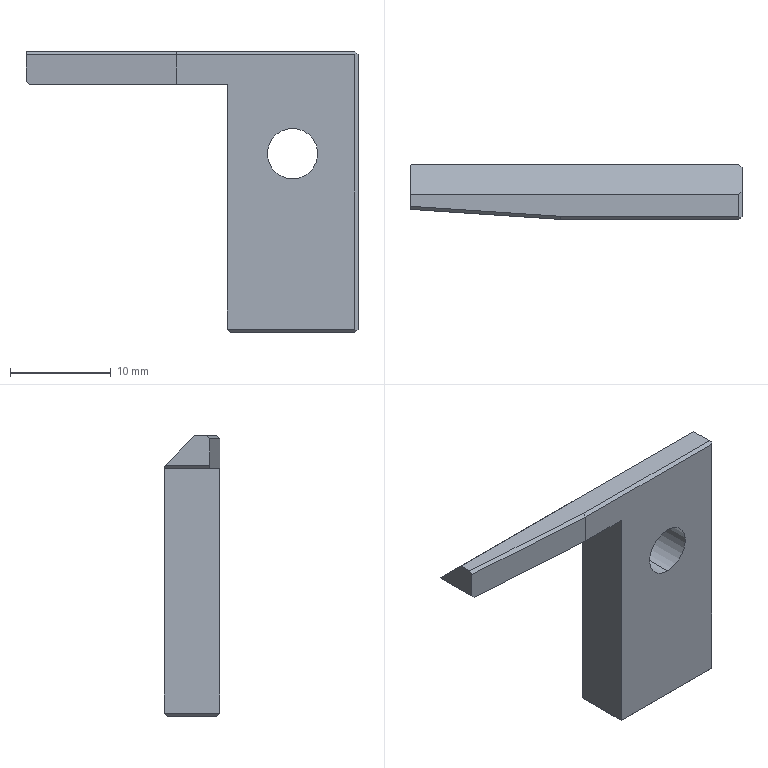Part | NX | 1 solid | 24 faces | box 33 x 5.5 x 27.85 mm | volume 2057 mm3 | plane 20 | cylinder 2 | cone 2 | commonest cylinder face diameters 5 x2
STEP:
#1=CARTESIAN_POINT('',(-176.3,222.248,-74.));
#2=VERTEX_POINT('',#1);
#3=CARTESIAN_POINT('',(-188.7,222.248,-74.));
#4=VERTEX_POINT('',#3);
#5=CARTESIAN_POINT('',(-182.5,222.248,-74.));
#6=DIRECTION('',(-1.,0.,0.));
#7=VECTOR('',#6,1000.);
#8=LINE('',#5,#7);
#9=EDGE_CURVE('',#2,#4,#8,.T.);
#10=ORIENTED_EDGE('',*,*,#9,.T.);
#11=CARTESIAN_POINT('',(-188.7,227.148,-74.));
#12=VERTEX_POINT('',#11);
#13=CARTESIAN_POINT('',(-188.7,224.698,-74.));
#14=DIRECTION('',(0.,-1.,0.));
#15=VECTOR('',#14,1000.);
#16=LINE('',#13,#15);
#17=EDGE_CURVE('',#12,#4,#16,.T.);
#18=ORIENTED_EDGE('',*,*,#17,.F.);
#19=CARTESIAN_POINT('',(-176.3,227.148,-74.));
#20=VERTEX_POINT('',#19);
#21=CARTESIAN_POINT('',(-182.5,227.148,-74.));
#22=DIRECTION('',(1.,0.,0.));
#23=VECTOR('',#22,1000.);
#24=LINE('',#21,#23);
#25=EDGE_CURVE('',#12,#20,#24,.T.);
#26=ORIENTED_EDGE('',*,*,#25,.T.);
#27=CARTESIAN_POINT('',(-176.3,224.698,-74.));
#28=DIRECTION('',(0.,-1.,0.));
#29=VECTOR('',#28,1000.);
#30=LINE('',#27,#29);
#31=EDGE_CURVE('',#20,#2,#30,.T.);
#32=ORIENTED_EDGE('',*,*,#31,.T.);
#33=EDGE_LOOP('',(#10,#18,#26,#32));
#34=FACE_BOUND('',#33,.T.);
#35=CARTESIAN_POINT('',(-175.,217.7,-74.));
#36=DIRECTION('',(0.,0.,-1.));
#37=DIRECTION('',(-1.,0.,0.));
#38=AXIS2_PLACEMENT_3D('',#35,#36,#37);
#39=PLANE('',#38);
#40=ADVANCED_FACE('',(#34),#39,.T.);
#41=CARTESIAN_POINT('',(-209.,227.348,-49.05));
#42=VERTEX_POINT('',#41);
#43=CARTESIAN_POINT('',(-209.,222.948,-49.05));
#44=VERTEX_POINT('',#43);
#45=CARTESIAN_POINT('',(-209.,225.198,-49.05));
#46=DIRECTION('',(0.,-1.,0.));
#47=VECTOR('',#46,1000.);
#48=LINE('',#45,#47);
#49=EDGE_CURVE('',#42,#44,#48,.T.);
#50=ORIENTED_EDGE('',*,*,#49,.T.);
#51=CARTESIAN_POINT('',(-209.,222.948,-46.45));
#52=VERTEX_POINT('',#51);
#53=CARTESIAN_POINT('',(-209.,222.948,-47.75));
#54=DIRECTION('',(0.,0.,-1.));
#55=VECTOR('',#54,1000.);
#56=LINE('',#53,#55);
#57=EDGE_CURVE('',#52,#44,#56,.T.);
#58=ORIENTED_EDGE('',*,*,#57,.F.);
#59=CARTESIAN_POINT('',(-209.,223.249,-46.15));
#60=VERTEX_POINT('',#59);
#61=CARTESIAN_POINT('',(-209.,213.364,-56.013));
#62=DIRECTION('',(0.,-0.7079,-0.7063));
#63=VECTOR('',#62,1000.);
#64=LINE('',#61,#63);
#65=EDGE_CURVE('',#60,#52,#64,.T.);
#66=ORIENTED_EDGE('',*,*,#65,.F.);
#67=CARTESIAN_POINT('',(-209.,224.448,-46.15));
#68=VERTEX_POINT('',#67);
#69=CARTESIAN_POINT('',(-209.,213.364,-46.15));
#70=DIRECTION('',(0.,1.,0.));
#71=VECTOR('',#70,1000.);
#72=LINE('',#69,#71);
#73=EDGE_CURVE('',#60,#68,#72,.T.);
#74=ORIENTED_EDGE('',*,*,#73,.T.);
#75=CARTESIAN_POINT('',(-209.,232.274,-53.975));
#76=DIRECTION('',(0.,0.7071,-0.7071));
#77=VECTOR('',#76,1000.);
#78=LINE('',#75,#77);
#79=EDGE_CURVE('',#68,#42,#78,.T.);
#80=ORIENTED_EDGE('',*,*,#79,.T.);
#81=EDGE_LOOP('',(#50,#58,#66,#74,#80));
#82=FACE_BOUND('',#81,.T.);
#83=CARTESIAN_POINT('',(-209.,224.834,-50.132));
#84=DIRECTION('',(-1.,0.,0.));
#85=DIRECTION('',(0.,0.,1.));
#86=AXIS2_PLACEMENT_3D('',#83,#84,#85);
#87=PLANE('',#86);
#88=ADVANCED_FACE('',(#82),#87,.T.);
#89=CARTESIAN_POINT('',(-176.3,227.448,-73.7));
#90=VERTEX_POINT('',#89);
#91=CARTESIAN_POINT('',(-176.3,227.448,-49.15));
#92=VERTEX_POINT('',#91);
#93=CARTESIAN_POINT('',(-176.3,227.448,-61.575));
#94=DIRECTION('',(0.,0.,1.));
#95=VECTOR('',#94,1000.);
#96=LINE('',#93,#95);
#97=EDGE_CURVE('',#90,#92,#96,.T.);
#98=ORIENTED_EDGE('',*,*,#97,.F.);
#99=CARTESIAN_POINT('',(-189.,227.448,-73.7));
#100=VERTEX_POINT('',#99);
#101=CARTESIAN_POINT('',(-182.5,227.448,-73.7));
#102=DIRECTION('',(1.,0.,0.));
#103=VECTOR('',#102,1000.);
#104=LINE('',#101,#103);
#105=EDGE_CURVE('',#100,#90,#104,.T.);
#106=ORIENTED_EDGE('',*,*,#105,.F.);
#107=CARTESIAN_POINT('',(-189.,227.448,-49.35));
#108=VERTEX_POINT('',#107);
#109=CARTESIAN_POINT('',(-189.,227.448,-53.975));
#110=DIRECTION('',(0.,0.,1.));
#111=VECTOR('',#110,1000.);
#112=LINE('',#109,#111);
#113=EDGE_CURVE('',#100,#108,#112,.T.);
#114=ORIENTED_EDGE('',*,*,#113,.T.);
#115=CARTESIAN_POINT('',(-208.7,227.448,-49.35));
#116=VERTEX_POINT('',#115);
#117=CARTESIAN_POINT('',(-175.,227.448,-49.35));
#118=DIRECTION('',(1.,0.,0.));
#119=VECTOR('',#118,1000.);
#120=LINE('',#117,#119);
#121=EDGE_CURVE('',#116,#108,#120,.T.);
#122=ORIENTED_EDGE('',*,*,#121,.F.);
#123=CARTESIAN_POINT('',(-208.9,227.448,-49.15));
#124=VERTEX_POINT('',#123);
#125=CARTESIAN_POINT('',(-204.075,227.448,-53.975));
#126=DIRECTION('',(0.7071,0.,-0.7071));
#127=VECTOR('',#126,1000.);
#128=LINE('',#125,#127);
#129=EDGE_CURVE('',#124,#116,#128,.T.);
#130=ORIENTED_EDGE('',*,*,#129,.F.);
#131=CARTESIAN_POINT('',(-192.5,227.448,-49.15));
#132=DIRECTION('',(1.,0.,0.));
#133=VECTOR('',#132,1000.);
#134=LINE('',#131,#133);
#135=EDGE_CURVE('',#124,#92,#134,.T.);
#136=ORIENTED_EDGE('',*,*,#135,.T.);
#137=EDGE_LOOP('',(#98,#106,#114,#122,#130,#136));
#138=FACE_BOUND('',#137,.T.);
#139=CARTESIAN_POINT('',(-182.5,227.448,-53.563));
#140=VERTEX_POINT('',#139);
#141=CARTESIAN_POINT('',(-182.5,227.448,-58.963));
#142=VERTEX_POINT('',#141);
#143=CARTESIAN_POINT('',(-182.5,227.448,-56.263));
#144=DIRECTION('',(0.,1.,0.));
#145=DIRECTION('',(0.,0.,-1.));
#146=AXIS2_PLACEMENT_3D('',#143,#144,#145);
#147=CIRCLE('',#146,2.7);
#148=EDGE_CURVE('',#140,#142,#147,.T.);
#149=ORIENTED_EDGE('',*,*,#148,.F.);
#150=CARTESIAN_POINT('',(-182.5,227.448,-56.263));
#151=DIRECTION('',(0.,1.,0.));
#152=DIRECTION('',(0.,0.,-1.));
#153=AXIS2_PLACEMENT_3D('',#150,#151,#152);
#154=CIRCLE('',#153,2.7);
#155=EDGE_CURVE('',#142,#140,#154,.T.);
#156=ORIENTED_EDGE('',*,*,#155,.F.);
#157=EDGE_LOOP('',(#149,#156));
#158=FACE_BOUND('',#157,.T.);
#159=CARTESIAN_POINT('',(-175.,227.448,-64.15));
#160=DIRECTION('',(0.,1.,0.));
#161=DIRECTION('',(0.,0.,-1.));
#162=AXIS2_PLACEMENT_3D('',#159,#160,#161);
#163=PLANE('',#162);
#164=ADVANCED_FACE('',(#138,#158),#163,.T.);
#165=CARTESIAN_POINT('',(-176.3,222.248,-46.15));
#166=VERTEX_POINT('',#165);
#167=CARTESIAN_POINT('',(-193.99,222.248,-46.15));
#168=VERTEX_POINT('',#167);
#169=CARTESIAN_POINT('',(-185.,222.248,-46.15));
#170=DIRECTION('',(-1.,0.,0.));
#171=VECTOR('',#170,1000.);
#172=LINE('',#169,#171);
#173=EDGE_CURVE('',#166,#168,#172,.T.);
#174=ORIENTED_EDGE('',*,*,#173,.F.);
#175=CARTESIAN_POINT('',(-176.3,224.448,-46.15));
#176=VERTEX_POINT('',#175);
#177=CARTESIAN_POINT('',(-176.3,223.198,-46.15));
#178=DIRECTION('',(0.,-1.,0.));
#179=VECTOR('',#178,1000.);
#180=LINE('',#177,#179);
#181=EDGE_CURVE('',#176,#166,#180,.T.);
#182=ORIENTED_EDGE('',*,*,#181,.F.);
#183=CARTESIAN_POINT('',(-192.5,224.448,-46.15));
#184=DIRECTION('',(1.,0.,0.));
#185=VECTOR('',#184,1000.);
#186=LINE('',#183,#185);
#187=EDGE_CURVE('',#68,#176,#186,.T.);
#188=ORIENTED_EDGE('',*,*,#187,.F.);
#189=ORIENTED_EDGE('',*,*,#73,.F.);
#190=CARTESIAN_POINT('',(-201.48,222.747,-46.15));
#191=DIRECTION('',(-0.9978,0.06652,0.));
#192=VECTOR('',#191,1000.);
#193=LINE('',#190,#192);
#194=EDGE_CURVE('',#168,#60,#193,.T.);
#195=ORIENTED_EDGE('',*,*,#194,.F.);
#196=EDGE_LOOP('',(#174,#182,#188,#189,#195));
#197=FACE_BOUND('',#196,.T.);
#198=CARTESIAN_POINT('',(-175.,222.398,-46.15));
#199=DIRECTION('',(0.,0.,1.));
#200=DIRECTION('',(1.,0.,0.));
#201=AXIS2_PLACEMENT_3D('',#198,#199,#200);
#202=PLANE('',#201);
#203=ADVANCED_FACE('',(#197),#202,.T.);
#204=CARTESIAN_POINT('',(-194.,221.948,-49.35));
#205=VERTEX_POINT('',#204);
#206=CARTESIAN_POINT('',(-189.,221.948,-49.35));
#207=VERTEX_POINT('',#206);
#208=CARTESIAN_POINT('',(-175.,221.948,-49.35));
#209=DIRECTION('',(1.,0.,0.));
#210=VECTOR('',#209,1000.);
#211=LINE('',#208,#210);
#212=EDGE_CURVE('',#205,#207,#211,.T.);
#213=ORIENTED_EDGE('',*,*,#212,.F.);
#214=CARTESIAN_POINT('',(-208.7,222.928,-49.35));
#215=VERTEX_POINT('',#214);
#216=CARTESIAN_POINT('',(-175.,220.681,-49.35));
#217=DIRECTION('',(0.9978,-0.06652,0.));
#218=VECTOR('',#217,1000.);
#219=LINE('',#216,#218);
#220=EDGE_CURVE('',#215,#205,#219,.T.);
#221=ORIENTED_EDGE('',*,*,#220,.F.);
#222=CARTESIAN_POINT('',(-208.7,225.198,-49.35));
#223=DIRECTION('',(0.,-1.,0.));
#224=VECTOR('',#223,1000.);
#225=LINE('',#222,#224);
#226=EDGE_CURVE('',#116,#215,#225,.T.);
#227=ORIENTED_EDGE('',*,*,#226,.F.);
#228=ORIENTED_EDGE('',*,*,#121,.T.);
#229=CARTESIAN_POINT('',(-189.,213.364,-49.35));
#230=DIRECTION('',(0.,1.,0.));
#231=VECTOR('',#230,1000.);
#232=LINE('',#229,#231);
#233=EDGE_CURVE('',#207,#108,#232,.T.);
#234=ORIENTED_EDGE('',*,*,#233,.F.);
#235=EDGE_LOOP('',(#213,#221,#227,#228,#234));
#236=FACE_BOUND('',#235,.T.);
#237=CARTESIAN_POINT('',(-189.,221.948,-49.35));
#238=DIRECTION('',(0.,0.,-1.));
#239=DIRECTION('',(-1.,0.,0.));
#240=AXIS2_PLACEMENT_3D('',#237,#238,#239);
#241=PLANE('',#240);
#242=ADVANCED_FACE('',(#236),#241,.T.);
#243=CARTESIAN_POINT('',(-176.3,221.948,-46.45));
#244=VERTEX_POINT('',#243);
#245=CARTESIAN_POINT('',(-194.,221.948,-46.45));
#246=VERTEX_POINT('',#245);
#247=CARTESIAN_POINT('',(-185.,221.948,-46.45));
#248=DIRECTION('',(-1.,0.,0.));
#249=VECTOR('',#248,1000.);
#250=LINE('',#247,#249);
#251=EDGE_CURVE('',#244,#246,#250,.T.);
#252=ORIENTED_EDGE('',*,*,#251,.T.);
#253=CARTESIAN_POINT('',(-194.,221.948,-47.75));
#254=DIRECTION('',(0.,0.,-1.));
#255=VECTOR('',#254,1000.);
#256=LINE('',#253,#255);
#257=EDGE_CURVE('',#246,#205,#256,.T.);
#258=ORIENTED_EDGE('',*,*,#257,.T.);
#259=ORIENTED_EDGE('',*,*,#212,.T.);
#260=CARTESIAN_POINT('',(-189.,221.948,-73.7));
#261=VERTEX_POINT('',#260);
#262=CARTESIAN_POINT('',(-189.,221.948,-53.975));
#263=DIRECTION('',(0.,0.,-1.));
#264=VECTOR('',#263,1000.);
#265=LINE('',#262,#264);
#266=EDGE_CURVE('',#207,#261,#265,.T.);
#267=ORIENTED_EDGE('',*,*,#266,.T.);
#268=CARTESIAN_POINT('',(-176.3,221.948,-73.7));
#269=VERTEX_POINT('',#268);
#270=CARTESIAN_POINT('',(-182.5,221.948,-73.7));
#271=DIRECTION('',(-1.,0.,0.));
#272=VECTOR('',#271,1000.);
#273=LINE('',#270,#272);
#274=EDGE_CURVE('',#269,#261,#273,.T.);
#275=ORIENTED_EDGE('',*,*,#274,.F.);
#276=CARTESIAN_POINT('',(-176.3,221.948,-60.075));
#277=DIRECTION('',(0.,0.,1.));
#278=VECTOR('',#277,1000.);
#279=LINE('',#276,#278);
#280=EDGE_CURVE('',#269,#244,#279,.T.);
#281=ORIENTED_EDGE('',*,*,#280,.T.);
#282=EDGE_LOOP('',(#252,#258,#259,#267,#275,#281));
#283=FACE_BOUND('',#282,.T.);
#284=CARTESIAN_POINT('',(-182.5,221.948,-53.763));
#285=VERTEX_POINT('',#284);
#286=CARTESIAN_POINT('',(-182.5,221.948,-58.763));
#287=VERTEX_POINT('',#286);
#288=CARTESIAN_POINT('',(-182.5,221.948,-56.263));
#289=DIRECTION('',(0.,1.,0.));
#290=DIRECTION('',(0.,0.,-1.));
#291=AXIS2_PLACEMENT_3D('',#288,#289,#290);
#292=CIRCLE('',#291,2.5);
#293=EDGE_CURVE('',#285,#287,#292,.T.);
#294=ORIENTED_EDGE('',*,*,#293,.T.);
#295=CARTESIAN_POINT('',(-182.5,221.948,-56.263));
#296=DIRECTION('',(0.,1.,0.));
#297=DIRECTION('',(0.,0.,-1.));
#298=AXIS2_PLACEMENT_3D('',#295,#296,#297);
#299=CIRCLE('',#298,2.5);
#300=EDGE_CURVE('',#287,#285,#299,.T.);
#301=ORIENTED_EDGE('',*,*,#300,.T.);
#302=EDGE_LOOP('',(#294,#301));
#303=FACE_BOUND('',#302,.T.);
#304=CARTESIAN_POINT('',(-189.,221.948,-45.15));
#305=DIRECTION('',(0.,-1.,0.));
#306=DIRECTION('',(-1.,0.,0.));
#307=AXIS2_PLACEMENT_3D('',#304,#305,#306);
#308=PLANE('',#307);
#309=ADVANCED_FACE('',(#283,#303),#308,.T.);
#310=CARTESIAN_POINT('',(-182.5,227.248,-53.763));
#311=VERTEX_POINT('',#310);
#312=CARTESIAN_POINT('',(-182.5,227.248,-58.763));
#313=VERTEX_POINT('',#312);
#314=CARTESIAN_POINT('',(-182.5,227.248,-56.263));
#315=DIRECTION('',(0.,1.,0.));
#316=DIRECTION('',(0.,0.,-1.));
#317=AXIS2_PLACEMENT_3D('',#314,#315,#316);
#318=CIRCLE('',#317,2.5);
#319=EDGE_CURVE('',#311,#313,#318,.T.);
#320=ORIENTED_EDGE('',*,*,#319,.T.);
#321=CARTESIAN_POINT('',(-182.5,227.948,-58.763));
#322=DIRECTION('',(0.,1.,0.));
#323=VECTOR('',#322,1000.);
#324=LINE('',#321,#323);
#325=EDGE_CURVE('',#313,#287,#324,.F.);
#326=ORIENTED_EDGE('',*,*,#325,.T.);
#327=ORIENTED_EDGE('',*,*,#293,.F.);
#328=CARTESIAN_POINT('',(-182.5,227.948,-53.763));
#329=DIRECTION('',(0.,1.,0.));
#330=VECTOR('',#329,1000.);
#331=LINE('',#328,#330);
#332=EDGE_CURVE('',#311,#285,#331,.F.);
#333=ORIENTED_EDGE('',*,*,#332,.F.);
#334=EDGE_LOOP('',(#320,#326,#327,#333));
#335=FACE_BOUND('',#334,.T.);
#336=CARTESIAN_POINT('',(-182.5,227.948,-56.263));
#337=DIRECTION('',(0.,1.,0.));
#338=DIRECTION('',(0.,0.,-1.));
#339=AXIS2_PLACEMENT_3D('',#336,#337,#338);
#340=CYLINDRICAL_SURFACE('',#339,2.5);
#341=ADVANCED_FACE('',(#335),#340,.F.);
#342=ORIENTED_EDGE('',*,*,#187,.T.);
#343=CARTESIAN_POINT('',(-176.,224.748,-46.45));
#344=VERTEX_POINT('',#343);
#345=CARTESIAN_POINT('',(-175.,225.748,-47.45));
#346=DIRECTION('',(0.5774,0.5774,-0.5774));
#347=VECTOR('',#346,1000.);
#348=LINE('',#345,#347);
#349=EDGE_CURVE('',#176,#344,#348,.T.);
#350=ORIENTED_EDGE('',*,*,#349,.T.);
#351=CARTESIAN_POINT('',(-176.,227.148,-48.85));
#352=VERTEX_POINT('',#351);
#353=CARTESIAN_POINT('',(-176.,232.274,-53.975));
#354=DIRECTION('',(0.,-0.7071,0.7071));
#355=VECTOR('',#354,1000.);
#356=LINE('',#353,#355);
#357=EDGE_CURVE('',#352,#344,#356,.T.);
#358=ORIENTED_EDGE('',*,*,#357,.F.);
#359=CARTESIAN_POINT('',(-181.125,232.274,-53.975));
#360=DIRECTION('',(-0.5774,0.5774,-0.5774));
#361=VECTOR('',#360,1000.);
#362=LINE('',#359,#361);
#363=EDGE_CURVE('',#352,#92,#362,.T.);
#364=ORIENTED_EDGE('',*,*,#363,.T.);
#365=ORIENTED_EDGE('',*,*,#135,.F.);
#366=CARTESIAN_POINT('',(-204.075,232.274,-53.975));
#367=DIRECTION('',(-0.5774,-0.5774,0.5774));
#368=VECTOR('',#367,1000.);
#369=LINE('',#366,#368);
#370=EDGE_CURVE('',#124,#42,#369,.T.);
#371=ORIENTED_EDGE('',*,*,#370,.T.);
#372=ORIENTED_EDGE('',*,*,#79,.F.);
#373=EDGE_LOOP('',(#342,#350,#358,#364,#365,#371,#372));
#374=FACE_BOUND('',#373,.T.);
#375=CARTESIAN_POINT('',(-192.5,225.948,-47.65));
#376=DIRECTION('',(0.,-0.7071,-0.7071));
#377=DIRECTION('',(0.,0.7071,-0.7071));
#378=AXIS2_PLACEMENT_3D('',#375,#376,#377);
#379=PLANE('',#378);
#380=ADVANCED_FACE('',(#374),#379,.F.);
#381=ORIENTED_EDGE('',*,*,#319,.F.);
#382=CARTESIAN_POINT('',(-182.5,227.248,-53.763));
#383=DIRECTION('',(0.,0.7071,0.7071));
#384=VECTOR('',#383,1000.);
#385=LINE('',#382,#384);
#386=EDGE_CURVE('',#140,#311,#385,.F.);
#387=ORIENTED_EDGE('',*,*,#386,.F.);
#388=ORIENTED_EDGE('',*,*,#148,.T.);
#389=CARTESIAN_POINT('',(-182.5,227.248,-58.763));
#390=DIRECTION('',(0.,0.7071,-0.7071));
#391=VECTOR('',#390,1000.);
#392=LINE('',#389,#391);
#393=EDGE_CURVE('',#142,#313,#392,.F.);
#394=ORIENTED_EDGE('',*,*,#393,.T.);
#395=EDGE_LOOP('',(#381,#387,#388,#394));
#396=FACE_BOUND('',#395,.T.);
#397=CARTESIAN_POINT('',(-182.5,227.248,-56.263));
#398=DIRECTION('',(0.,1.,0.));
#399=DIRECTION('',(0.,0.,-1.));
#400=AXIS2_PLACEMENT_3D('',#397,#398,#399);
#401=CONICAL_SURFACE('',#400,2.5,0.7854);
#402=ADVANCED_FACE('',(#396),#401,.F.);
#403=CARTESIAN_POINT('',(-201.5,222.448,-46.45));
#404=DIRECTION('',(-0.9978,0.06652,0.));
#405=VECTOR('',#404,1000.);
#406=LINE('',#403,#405);
#407=EDGE_CURVE('',#246,#52,#406,.T.);
#408=ORIENTED_EDGE('',*,*,#407,.T.);
#409=ORIENTED_EDGE('',*,*,#57,.T.);
#410=CARTESIAN_POINT('',(-204.075,222.62,-53.975));
#411=DIRECTION('',(-0.7063,0.04709,0.7063));
#412=VECTOR('',#411,1000.);
#413=LINE('',#410,#412);
#414=EDGE_CURVE('',#215,#44,#413,.T.);
#415=ORIENTED_EDGE('',*,*,#414,.F.);
#416=ORIENTED_EDGE('',*,*,#220,.T.);
#417=ORIENTED_EDGE('',*,*,#257,.F.);
#418=EDGE_LOOP('',(#408,#409,#415,#416,#417));
#419=FACE_BOUND('',#418,.T.);
#420=CARTESIAN_POINT('',(-201.5,222.448,-47.75));
#421=DIRECTION('',(-0.06652,-0.9978,0.));
#422=DIRECTION('',(-0.9978,0.06652,0.));
#423=AXIS2_PLACEMENT_3D('',#420,#421,#422);
#424=PLANE('',#423);
#425=ADVANCED_FACE('',(#419),#424,.T.);
#426=ORIENTED_EDGE('',*,*,#25,.F.);
#427=CARTESIAN_POINT('',(-174.916,213.364,-87.784));
#428=DIRECTION('',(-0.5774,0.5774,0.5774));
#429=VECTOR('',#428,1000.);
#430=LINE('',#427,#429);
#431=EDGE_CURVE('',#12,#100,#430,.T.);
#432=ORIENTED_EDGE('',*,*,#431,.T.);
#433=ORIENTED_EDGE('',*,*,#105,.T.);
#434=CARTESIAN_POINT('',(-176.15,227.298,-73.85));
#435=VERTEX_POINT('',#434);
#436=CARTESIAN_POINT('',(-162.216,213.364,-87.784));
#437=DIRECTION('',(-0.5774,0.5774,0.5774));
#438=VECTOR('',#437,1000.);
#439=LINE('',#436,#438);
#440=EDGE_CURVE('',#435,#90,#439,.T.);
#441=ORIENTED_EDGE('',*,*,#440,.F.);
#442=CARTESIAN_POINT('',(-190.084,213.364,-87.784));
#443=DIRECTION('',(0.5774,0.5774,0.5774));
#444=VECTOR('',#443,1000.);
#445=LINE('',#442,#444);
#446=EDGE_CURVE('',#20,#435,#445,.T.);
#447=ORIENTED_EDGE('',*,*,#446,.F.);
#448=EDGE_LOOP('',(#426,#432,#433,#441,#447));
#449=FACE_BOUND('',#448,.T.);
#450=CARTESIAN_POINT('',(-182.5,227.298,-73.85));
#451=DIRECTION('',(0.,0.7071,-0.7071));
#452=DIRECTION('',(-1.,0.,0.));
#453=AXIS2_PLACEMENT_3D('',#450,#451,#452);
#454=PLANE('',#453);
#455=ADVANCED_FACE('',(#449),#454,.T.);
#456=ORIENTED_EDGE('',*,*,#9,.F.);
#457=CARTESIAN_POINT('',(-176.15,222.098,-73.85));
#458=VERTEX_POINT('',#457);
#459=CARTESIAN_POINT('',(-167.416,213.364,-65.116));
#460=DIRECTION('',(0.5774,-0.5774,0.5774));
#461=VECTOR('',#460,1000.);
#462=LINE('',#459,#461);
#463=EDGE_CURVE('',#2,#458,#462,.T.);
#464=ORIENTED_EDGE('',*,*,#463,.T.);
#465=CARTESIAN_POINT('',(-184.884,213.364,-65.116));
#466=DIRECTION('',(0.5774,0.5774,-0.5774));
#467=VECTOR('',#466,1000.);
#468=LINE('',#465,#467);
#469=EDGE_CURVE('',#269,#458,#468,.T.);
#470=ORIENTED_EDGE('',*,*,#469,.F.);
#471=ORIENTED_EDGE('',*,*,#274,.T.);
#472=CARTESIAN_POINT('',(-197.584,213.364,-65.116));
#473=DIRECTION('',(0.5774,0.5774,-0.5774));
#474=VECTOR('',#473,1000.);
#475=LINE('',#472,#474);
#476=EDGE_CURVE('',#261,#4,#475,.T.);
#477=ORIENTED_EDGE('',*,*,#476,.T.);
#478=EDGE_LOOP('',(#456,#464,#470,#471,#477));
#479=FACE_BOUND('',#478,.T.);
#480=CARTESIAN_POINT('',(-182.5,222.098,-73.85));
#481=DIRECTION('',(0.,-0.7071,-0.7071));
#482=DIRECTION('',(0.,-0.7071,0.7071));
#483=AXIS2_PLACEMENT_3D('',#480,#481,#482);
#484=PLANE('',#483);
#485=ADVANCED_FACE('',(#479),#484,.T.);
#486=ORIENTED_EDGE('',*,*,#49,.F.);
#487=ORIENTED_EDGE('',*,*,#370,.F.);
#488=ORIENTED_EDGE('',*,*,#129,.T.);
#489=ORIENTED_EDGE('',*,*,#226,.T.);
#490=ORIENTED_EDGE('',*,*,#414,.T.);
#491=EDGE_LOOP('',(#486,#487,#488,#489,#490));
#492=FACE_BOUND('',#491,.T.);
#493=CARTESIAN_POINT('',(-208.85,225.198,-49.2));
#494=DIRECTION('',(-0.7071,0.,-0.7071));
#495=DIRECTION('',(-0.7071,0.,0.7071));
#496=AXIS2_PLACEMENT_3D('',#493,#494,#495);
#497=PLANE('',#496);
#498=ADVANCED_FACE('',(#492),#497,.T.);
#499=ORIENTED_EDGE('',*,*,#251,.F.);
#500=CARTESIAN_POINT('',(-176.15,222.098,-46.3));
#501=VERTEX_POINT('',#500);
#502=CARTESIAN_POINT('',(-175.,223.248,-45.15));
#503=DIRECTION('',(0.5774,0.5774,0.5774));
#504=VECTOR('',#503,1000.);
#505=LINE('',#502,#504);
#506=EDGE_CURVE('',#244,#501,#505,.T.);
#507=ORIENTED_EDGE('',*,*,#506,.T.);
#508=CARTESIAN_POINT('',(-167.416,213.364,-55.034));
#509=DIRECTION('',(-0.5774,0.5774,0.5774));
#510=VECTOR('',#509,1000.);
#511=LINE('',#508,#510);
#512=EDGE_CURVE('',#501,#166,#511,.T.);
#513=ORIENTED_EDGE('',*,*,#512,.T.);
#514=ORIENTED_EDGE('',*,*,#173,.T.);
#515=CARTESIAN_POINT('',(-194.286,213.364,-55.034));
#516=DIRECTION('',(-0.02354,-0.7069,-0.7069));
#517=VECTOR('',#516,1000.);
#518=LINE('',#515,#517);
#519=EDGE_CURVE('',#168,#246,#518,.T.);
#520=ORIENTED_EDGE('',*,*,#519,.T.);
#521=EDGE_LOOP('',(#499,#507,#513,#514,#520));
#522=FACE_BOUND('',#521,.T.);
#523=CARTESIAN_POINT('',(-185.,222.098,-46.3));
#524=DIRECTION('',(0.,-0.7071,0.7071));
#525=DIRECTION('',(-1.,0.,0.));
#526=AXIS2_PLACEMENT_3D('',#523,#524,#525);
#527=PLANE('',#526);
#528=ADVANCED_FACE('',(#522),#527,.T.);
#529=ORIENTED_EDGE('',*,*,#407,.F.);
#530=ORIENTED_EDGE('',*,*,#519,.F.);
#531=ORIENTED_EDGE('',*,*,#194,.T.);
#532=ORIENTED_EDGE('',*,*,#65,.T.);
#533=EDGE_LOOP('',(#529,#530,#531,#532));
#534=FACE_BOUND('',#533,.T.);
#535=CARTESIAN_POINT('',(-201.49,222.598,-46.3));
#536=DIRECTION('',(-0.04704,-0.7055,0.7071));
#537=DIRECTION('',(-0.9978,0.06652,0.));
#538=AXIS2_PLACEMENT_3D('',#535,#536,#537);
#539=PLANE('',#538);
#540=ADVANCED_FACE('',(#534),#539,.T.);
#541=ORIENTED_EDGE('',*,*,#393,.F.);
#542=ORIENTED_EDGE('',*,*,#155,.T.);
#543=ORIENTED_EDGE('',*,*,#386,.T.);
#544=CARTESIAN_POINT('',(-182.5,227.248,-56.263));
#545=DIRECTION('',(0.,1.,0.));
#546=DIRECTION('',(0.,0.,-1.));
#547=AXIS2_PLACEMENT_3D('',#544,#545,#546);
#548=CIRCLE('',#547,2.5);
#549=EDGE_CURVE('',#313,#311,#548,.T.);
#550=ORIENTED_EDGE('',*,*,#549,.F.);
#551=EDGE_LOOP('',(#541,#542,#543,#550));
#552=FACE_BOUND('',#551,.T.);
#553=CARTESIAN_POINT('',(-182.5,227.248,-56.263));
#554=DIRECTION('',(0.,1.,0.));
#555=DIRECTION('',(0.,0.,-1.));
#556=AXIS2_PLACEMENT_3D('',#553,#554,#555);
#557=CONICAL_SURFACE('',#556,2.5,0.7854);
#558=ADVANCED_FACE('',(#552),#557,.F.);
#559=ORIENTED_EDGE('',*,*,#325,.F.);
#560=ORIENTED_EDGE('',*,*,#549,.T.);
#561=ORIENTED_EDGE('',*,*,#332,.T.);
#562=ORIENTED_EDGE('',*,*,#300,.F.);
#563=EDGE_LOOP('',(#559,#560,#561,#562));
#564=FACE_BOUND('',#563,.T.);
#565=CARTESIAN_POINT('',(-182.5,227.948,-56.263));
#566=DIRECTION('',(0.,1.,0.));
#567=DIRECTION('',(0.,0.,-1.));
#568=AXIS2_PLACEMENT_3D('',#565,#566,#567);
#569=CYLINDRICAL_SURFACE('',#568,2.5);
#570=ADVANCED_FACE('',(#564),#569,.F.);
#571=CARTESIAN_POINT('',(-189.,224.698,-73.7));
#572=DIRECTION('',(0.,-1.,0.));
#573=VECTOR('',#572,1000.);
#574=LINE('',#571,#573);
#575=EDGE_CURVE('',#100,#261,#574,.T.);
#576=ORIENTED_EDGE('',*,*,#575,.T.);
#577=ORIENTED_EDGE('',*,*,#266,.F.);
#578=ORIENTED_EDGE('',*,*,#233,.T.);
#579=ORIENTED_EDGE('',*,*,#113,.F.);
#580=EDGE_LOOP('',(#576,#577,#578,#579));
#581=FACE_BOUND('',#580,.T.);
#582=CARTESIAN_POINT('',(-189.,213.364,-53.975));
#583=DIRECTION('',(1.,0.,0.));
#584=DIRECTION('',(0.,-1.,0.));
#585=AXIS2_PLACEMENT_3D('',#582,#583,#584);
#586=PLANE('',#585);
#587=ADVANCED_FACE('',(#581),#586,.F.);
#588=ORIENTED_EDGE('',*,*,#575,.F.);
#589=ORIENTED_EDGE('',*,*,#431,.F.);
#590=ORIENTED_EDGE('',*,*,#17,.T.);
#591=ORIENTED_EDGE('',*,*,#476,.F.);
#592=EDGE_LOOP('',(#588,#589,#590,#591));
#593=FACE_BOUND('',#592,.T.);
#594=CARTESIAN_POINT('',(-188.85,224.698,-73.85));
#595=DIRECTION('',(-0.7071,0.,-0.7071));
#596=DIRECTION('',(-0.7071,0.,0.7071));
#597=AXIS2_PLACEMENT_3D('',#594,#595,#596);
#598=PLANE('',#597);
#599=ADVANCED_FACE('',(#593),#598,.T.);
#600=CARTESIAN_POINT('',(-176.,222.248,-46.45));
#601=VERTEX_POINT('',#600);
#602=CARTESIAN_POINT('',(-176.,223.198,-46.45));
#603=DIRECTION('',(0.,-1.,0.));
#604=VECTOR('',#603,1000.);
#605=LINE('',#602,#604);
#606=EDGE_CURVE('',#344,#601,#605,.T.);
#607=ORIENTED_EDGE('',*,*,#606,.T.);
#608=CARTESIAN_POINT('',(-176.,222.248,-73.7));
#609=VERTEX_POINT('',#608);
#610=CARTESIAN_POINT('',(-176.,222.248,-60.075));
#611=DIRECTION('',(0.,0.,1.));
#612=VECTOR('',#611,1000.);
#613=LINE('',#610,#612);
#614=EDGE_CURVE('',#609,#601,#613,.T.);
#615=ORIENTED_EDGE('',*,*,#614,.F.);
#616=CARTESIAN_POINT('',(-176.,227.148,-73.7));
#617=VERTEX_POINT('',#616);
#618=CARTESIAN_POINT('',(-176.,224.698,-73.7));
#619=DIRECTION('',(0.,-1.,0.));
#620=VECTOR('',#619,1000.);
#621=LINE('',#618,#620);
#622=EDGE_CURVE('',#617,#609,#621,.T.);
#623=ORIENTED_EDGE('',*,*,#622,.F.);
#624=CARTESIAN_POINT('',(-176.,227.148,-61.575));
#625=DIRECTION('',(0.,0.,1.));
#626=VECTOR('',#625,1000.);
#627=LINE('',#624,#626);
#628=EDGE_CURVE('',#617,#352,#627,.T.);
#629=ORIENTED_EDGE('',*,*,#628,.T.);
#630=ORIENTED_EDGE('',*,*,#357,.T.);
#631=EDGE_LOOP('',(#607,#615,#623,#629,#630));
#632=FACE_BOUND('',#631,.T.);
#633=CARTESIAN_POINT('',(-176.,213.364,-53.975));
#634=DIRECTION('',(1.,0.,0.));
#635=DIRECTION('',(0.,-1.,0.));
#636=AXIS2_PLACEMENT_3D('',#633,#634,#635);
#637=PLANE('',#636);
#638=ADVANCED_FACE('',(#632),#637,.T.);
#639=ORIENTED_EDGE('',*,*,#628,.F.);
#640=CARTESIAN_POINT('',(-156.275,207.424,-53.975));
#641=DIRECTION('',(0.5774,-0.5774,0.5774));
#642=VECTOR('',#641,1000.);
#643=LINE('',#640,#642);
#644=EDGE_CURVE('',#435,#617,#643,.T.);
#645=ORIENTED_EDGE('',*,*,#644,.F.);
#646=ORIENTED_EDGE('',*,*,#440,.T.);
#647=ORIENTED_EDGE('',*,*,#97,.T.);
#648=ORIENTED_EDGE('',*,*,#363,.F.);
#649=EDGE_LOOP('',(#639,#645,#646,#647,#648));
#650=FACE_BOUND('',#649,.T.);
#651=CARTESIAN_POINT('',(-176.15,227.298,-61.575));
#652=DIRECTION('',(0.7071,0.7071,0.));
#653=DIRECTION('',(0.,0.,-1.));
#654=AXIS2_PLACEMENT_3D('',#651,#652,#653);
#655=PLANE('',#654);
#656=ADVANCED_FACE('',(#650),#655,.T.);
#657=ORIENTED_EDGE('',*,*,#622,.T.);
#658=CARTESIAN_POINT('',(-156.275,241.973,-53.975));
#659=DIRECTION('',(-0.5774,-0.5774,-0.5774));
#660=VECTOR('',#659,1000.);
#661=LINE('',#658,#660);
#662=EDGE_CURVE('',#609,#458,#661,.T.);
#663=ORIENTED_EDGE('',*,*,#662,.T.);
#664=ORIENTED_EDGE('',*,*,#463,.F.);
#665=ORIENTED_EDGE('',*,*,#31,.F.);
#666=ORIENTED_EDGE('',*,*,#446,.T.);
#667=ORIENTED_EDGE('',*,*,#644,.T.);
#668=EDGE_LOOP('',(#657,#663,#664,#665,#666,#667));
#669=FACE_BOUND('',#668,.T.);
#670=CARTESIAN_POINT('',(-176.15,224.698,-73.85));
#671=DIRECTION('',(-0.7071,0.,0.7071));
#672=DIRECTION('',(0.,1.,0.));
#673=AXIS2_PLACEMENT_3D('',#670,#671,#672);
#674=PLANE('',#673);
#675=ADVANCED_FACE('',(#669),#674,.F.);
#676=ORIENTED_EDGE('',*,*,#614,.T.);
#677=CARTESIAN_POINT('',(-175.,223.248,-47.45));
#678=DIRECTION('',(0.5774,0.5774,-0.5774));
#679=VECTOR('',#678,1000.);
#680=LINE('',#677,#679);
#681=EDGE_CURVE('',#501,#601,#680,.T.);
#682=ORIENTED_EDGE('',*,*,#681,.F.);
#683=ORIENTED_EDGE('',*,*,#506,.F.);
#684=ORIENTED_EDGE('',*,*,#280,.F.);
#685=ORIENTED_EDGE('',*,*,#469,.T.);
#686=ORIENTED_EDGE('',*,*,#662,.F.);
#687=EDGE_LOOP('',(#676,#682,#683,#684,#685,#686));
#688=FACE_BOUND('',#687,.T.);
#689=CARTESIAN_POINT('',(-176.15,222.098,-60.075));
#690=DIRECTION('',(-0.7071,0.7071,0.));
#691=DIRECTION('',(0.,0.,1.));
#692=AXIS2_PLACEMENT_3D('',#689,#690,#691);
#693=PLANE('',#692);
#694=ADVANCED_FACE('',(#688),#693,.F.);
#695=ORIENTED_EDGE('',*,*,#606,.F.);
#696=ORIENTED_EDGE('',*,*,#349,.F.);
#697=ORIENTED_EDGE('',*,*,#181,.T.);
#698=ORIENTED_EDGE('',*,*,#512,.F.);
#699=ORIENTED_EDGE('',*,*,#681,.T.);
#700=EDGE_LOOP('',(#695,#696,#697,#698,#699));
#701=FACE_BOUND('',#700,.T.);
#702=CARTESIAN_POINT('',(-176.15,223.198,-46.3));
#703=DIRECTION('',(0.7071,0.,0.7071));
#704=DIRECTION('',(0.,-1.,0.));
#705=AXIS2_PLACEMENT_3D('',#702,#703,#704);
#706=PLANE('',#705);
#707=ADVANCED_FACE('',(#701),#706,.T.);
#708=CLOSED_SHELL('',(#40,#88,#164,#203,#242,#309,#341,#380,#402,#425,#455,#485,#498,#528,#540,#558,#570,#587,#599,#638,#656,#675,#694,#707));
#709=MANIFOLD_SOLID_BREP('',#708);
#710=(LENGTH_UNIT()NAMED_UNIT(*)SI_UNIT(.MILLI.,.METRE.));
#711=UNCERTAINTY_MEASURE_WITH_UNIT(LENGTH_MEASURE(0.00001),#710,'','');
#712=(NAMED_UNIT(*)PLANE_ANGLE_UNIT()SI_UNIT($,.RADIAN.));
#713=(NAMED_UNIT(*)SI_UNIT($,.STERADIAN.)SOLID_ANGLE_UNIT());
#714=(GEOMETRIC_REPRESENTATION_CONTEXT(3)GLOBAL_UNCERTAINTY_ASSIGNED_CONTEXT((#711))GLOBAL_UNIT_ASSIGNED_CONTEXT((#710,#712,#713))REPRESENTATION_CONTEXT('',''));
#715=ADVANCED_BREP_SHAPE_REPRESENTATION('',(#709),#714);